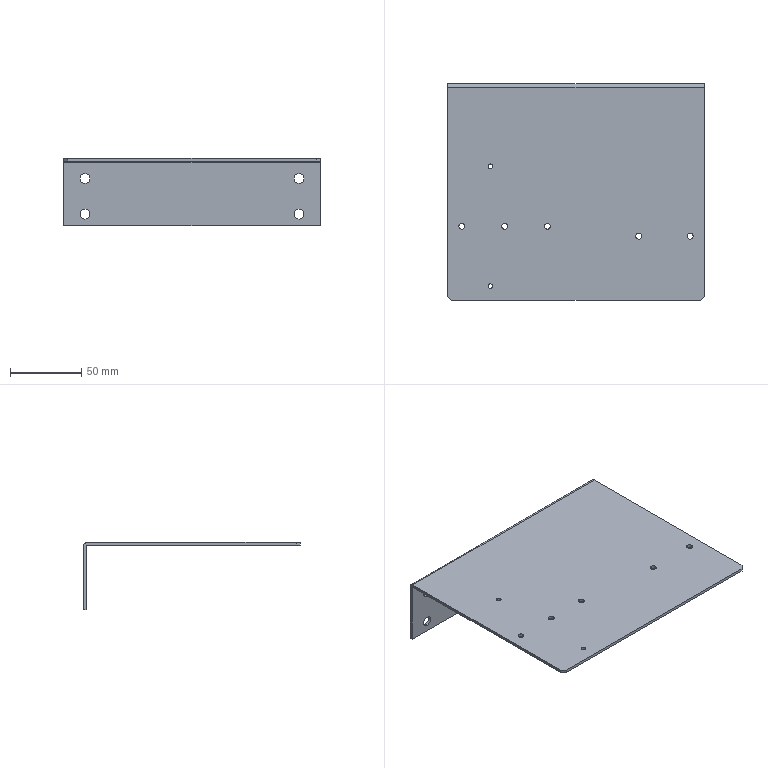Part | SolidWorks | features BaseBody 1 | 1 solid | 34 faces | box 180 x 152 x 47 mm | volume 70153 mm3 | cylinder 24 | plane 10 | commonest cylinder face diameters 4.2 x10 7 x8 3.3 x4 1.473 x1 5.473 x1
STEP:
#1=CARTESIAN_POINT('',(-80.,-100.1,2.));
#2=VERTEX_POINT('',#1);
#3=CARTESIAN_POINT('',(-80.,-95.9,2.));
#4=VERTEX_POINT('',#3);
#5=CARTESIAN_POINT('',(-80.,-98.,2.));
#6=DIRECTION('',(0.,0.,-1.));
#7=DIRECTION('',(0.,1.,0.));
#8=AXIS2_PLACEMENT_3D('',#5,#6,#7);
#9=CIRCLE('',#8,2.1);
#10=EDGE_CURVE('',#2,#4,#9,.T.);
#11=ORIENTED_EDGE('',*,*,#10,.F.);
#12=CARTESIAN_POINT('',(-80.,-100.1,0.));
#13=VERTEX_POINT('',#12);
#14=CARTESIAN_POINT('',(-80.,-100.1,0.));
#15=DIRECTION('',(0.,0.,-1.));
#16=VECTOR('',#15,1000.);
#17=LINE('',#14,#16);
#18=EDGE_CURVE('',#2,#13,#17,.T.);
#19=ORIENTED_EDGE('',*,*,#18,.T.);
#20=CARTESIAN_POINT('',(-80.,-95.9,0.));
#21=VERTEX_POINT('',#20);
#22=CARTESIAN_POINT('',(-80.,-98.,0.));
#23=DIRECTION('',(0.,0.,-1.));
#24=DIRECTION('',(0.,1.,0.));
#25=AXIS2_PLACEMENT_3D('',#22,#23,#24);
#26=CIRCLE('',#25,2.1);
#27=EDGE_CURVE('',#13,#21,#26,.T.);
#28=ORIENTED_EDGE('',*,*,#27,.T.);
#29=CARTESIAN_POINT('',(-80.,-95.9,0.));
#30=DIRECTION('',(0.,0.,-1.));
#31=VECTOR('',#30,1000.);
#32=LINE('',#29,#31);
#33=EDGE_CURVE('',#4,#21,#32,.T.);
#34=ORIENTED_EDGE('',*,*,#33,.F.);
#35=EDGE_LOOP('',(#11,#19,#28,#34));
#36=FACE_OUTER_BOUND('',#35,.T.);
#37=CARTESIAN_POINT('',(-80.,-98.,0.));
#38=DIRECTION('',(0.,0.,-1.));
#39=DIRECTION('',(0.,1.,0.));
#40=AXIS2_PLACEMENT_3D('',#37,#38,#39);
#41=CYLINDRICAL_SURFACE('',#40,2.1);
#42=ADVANCED_FACE('',(#36),#41,.F.);
#43=CARTESIAN_POINT('',(-50.,-100.1,2.));
#44=VERTEX_POINT('',#43);
#45=CARTESIAN_POINT('',(-50.,-95.9,2.));
#46=VERTEX_POINT('',#45);
#47=CARTESIAN_POINT('',(-50.,-98.,2.));
#48=DIRECTION('',(0.,0.,-1.));
#49=DIRECTION('',(0.,1.,0.));
#50=AXIS2_PLACEMENT_3D('',#47,#48,#49);
#51=CIRCLE('',#50,2.1);
#52=EDGE_CURVE('',#44,#46,#51,.T.);
#53=ORIENTED_EDGE('',*,*,#52,.F.);
#54=CARTESIAN_POINT('',(-50.,-100.1,0.));
#55=VERTEX_POINT('',#54);
#56=CARTESIAN_POINT('',(-50.,-100.1,0.));
#57=DIRECTION('',(0.,0.,-1.));
#58=VECTOR('',#57,1000.);
#59=LINE('',#56,#58);
#60=EDGE_CURVE('',#44,#55,#59,.T.);
#61=ORIENTED_EDGE('',*,*,#60,.T.);
#62=CARTESIAN_POINT('',(-50.,-95.9,0.));
#63=VERTEX_POINT('',#62);
#64=CARTESIAN_POINT('',(-50.,-98.,0.));
#65=DIRECTION('',(0.,0.,-1.));
#66=DIRECTION('',(0.,1.,0.));
#67=AXIS2_PLACEMENT_3D('',#64,#65,#66);
#68=CIRCLE('',#67,2.1);
#69=EDGE_CURVE('',#55,#63,#68,.T.);
#70=ORIENTED_EDGE('',*,*,#69,.T.);
#71=CARTESIAN_POINT('',(-50.,-95.9,0.));
#72=DIRECTION('',(0.,0.,-1.));
#73=VECTOR('',#72,1000.);
#74=LINE('',#71,#73);
#75=EDGE_CURVE('',#46,#63,#74,.T.);
#76=ORIENTED_EDGE('',*,*,#75,.F.);
#77=EDGE_LOOP('',(#53,#61,#70,#76));
#78=FACE_OUTER_BOUND('',#77,.T.);
#79=CARTESIAN_POINT('',(-50.,-98.,0.));
#80=DIRECTION('',(0.,0.,-1.));
#81=DIRECTION('',(0.,1.,0.));
#82=AXIS2_PLACEMENT_3D('',#79,#80,#81);
#83=CYLINDRICAL_SURFACE('',#82,2.1);
#84=ADVANCED_FACE('',(#78),#83,.F.);
#85=CARTESIAN_POINT('',(-20.,-100.1,2.));
#86=VERTEX_POINT('',#85);
#87=CARTESIAN_POINT('',(-20.,-95.9,2.));
#88=VERTEX_POINT('',#87);
#89=CARTESIAN_POINT('',(-20.,-98.,2.));
#90=DIRECTION('',(0.,0.,-1.));
#91=DIRECTION('',(0.,1.,0.));
#92=AXIS2_PLACEMENT_3D('',#89,#90,#91);
#93=CIRCLE('',#92,2.1);
#94=EDGE_CURVE('',#86,#88,#93,.T.);
#95=ORIENTED_EDGE('',*,*,#94,.F.);
#96=CARTESIAN_POINT('',(-20.,-100.1,0.));
#97=VERTEX_POINT('',#96);
#98=CARTESIAN_POINT('',(-20.,-100.1,0.));
#99=DIRECTION('',(0.,0.,-1.));
#100=VECTOR('',#99,1000.);
#101=LINE('',#98,#100);
#102=EDGE_CURVE('',#86,#97,#101,.T.);
#103=ORIENTED_EDGE('',*,*,#102,.T.);
#104=CARTESIAN_POINT('',(-20.,-95.9,0.));
#105=VERTEX_POINT('',#104);
#106=CARTESIAN_POINT('',(-20.,-98.,0.));
#107=DIRECTION('',(0.,0.,-1.));
#108=DIRECTION('',(0.,1.,0.));
#109=AXIS2_PLACEMENT_3D('',#106,#107,#108);
#110=CIRCLE('',#109,2.1);
#111=EDGE_CURVE('',#97,#105,#110,.T.);
#112=ORIENTED_EDGE('',*,*,#111,.T.);
#113=CARTESIAN_POINT('',(-20.,-95.9,0.));
#114=DIRECTION('',(0.,0.,-1.));
#115=VECTOR('',#114,1000.);
#116=LINE('',#113,#115);
#117=EDGE_CURVE('',#88,#105,#116,.T.);
#118=ORIENTED_EDGE('',*,*,#117,.F.);
#119=EDGE_LOOP('',(#95,#103,#112,#118));
#120=FACE_OUTER_BOUND('',#119,.T.);
#121=CARTESIAN_POINT('',(-20.,-98.,0.));
#122=DIRECTION('',(0.,0.,-1.));
#123=DIRECTION('',(0.,1.,0.));
#124=AXIS2_PLACEMENT_3D('',#121,#122,#123);
#125=CYLINDRICAL_SURFACE('',#124,2.1);
#126=ADVANCED_FACE('',(#120),#125,.F.);
#127=CARTESIAN_POINT('',(75.,0.,-33.5));
#128=VERTEX_POINT('',#127);
#129=CARTESIAN_POINT('',(75.,0.,-40.5));
#130=VERTEX_POINT('',#129);
#131=CARTESIAN_POINT('',(75.,0.,-37.));
#132=DIRECTION('',(0.,-1.,0.));
#133=DIRECTION('',(0.,0.,-1.));
#134=AXIS2_PLACEMENT_3D('',#131,#132,#133);
#135=CIRCLE('',#134,3.5);
#136=EDGE_CURVE('',#128,#130,#135,.T.);
#137=ORIENTED_EDGE('',*,*,#136,.T.);
#138=CARTESIAN_POINT('',(75.,2.,-40.5));
#139=VERTEX_POINT('',#138);
#140=CARTESIAN_POINT('',(75.,-8.,-40.5));
#141=DIRECTION('',(0.,1.,0.));
#142=VECTOR('',#141,1000.);
#143=LINE('',#140,#142);
#144=EDGE_CURVE('',#130,#139,#143,.T.);
#145=ORIENTED_EDGE('',*,*,#144,.T.);
#146=CARTESIAN_POINT('',(75.,2.,-33.5));
#147=VERTEX_POINT('',#146);
#148=CARTESIAN_POINT('',(75.,2.,-37.));
#149=DIRECTION('',(0.,1.,0.));
#150=DIRECTION('',(0.,0.,-1.));
#151=AXIS2_PLACEMENT_3D('',#148,#149,#150);
#152=CIRCLE('',#151,3.5);
#153=EDGE_CURVE('',#139,#147,#152,.T.);
#154=ORIENTED_EDGE('',*,*,#153,.T.);
#155=CARTESIAN_POINT('',(75.,-8.,-33.5));
#156=DIRECTION('',(0.,1.,0.));
#157=VECTOR('',#156,1000.);
#158=LINE('',#155,#157);
#159=EDGE_CURVE('',#128,#147,#158,.T.);
#160=ORIENTED_EDGE('',*,*,#159,.F.);
#161=EDGE_LOOP('',(#137,#145,#154,#160));
#162=FACE_OUTER_BOUND('',#161,.T.);
#163=CARTESIAN_POINT('',(75.,-8.,-37.));
#164=DIRECTION('',(0.,1.,0.));
#165=DIRECTION('',(0.,0.,1.));
#166=AXIS2_PLACEMENT_3D('',#163,#164,#165);
#167=CYLINDRICAL_SURFACE('',#166,3.5);
#168=ADVANCED_FACE('',(#162),#167,.F.);
#169=CARTESIAN_POINT('',(75.,0.,-8.5));
#170=VERTEX_POINT('',#169);
#171=CARTESIAN_POINT('',(75.,0.,-15.5));
#172=VERTEX_POINT('',#171);
#173=CARTESIAN_POINT('',(75.,0.,-12.));
#174=DIRECTION('',(0.,-1.,0.));
#175=DIRECTION('',(0.,0.,-1.));
#176=AXIS2_PLACEMENT_3D('',#173,#174,#175);
#177=CIRCLE('',#176,3.5);
#178=EDGE_CURVE('',#170,#172,#177,.T.);
#179=ORIENTED_EDGE('',*,*,#178,.T.);
#180=CARTESIAN_POINT('',(75.,2.,-15.5));
#181=VERTEX_POINT('',#180);
#182=CARTESIAN_POINT('',(75.,-8.,-15.5));
#183=DIRECTION('',(0.,1.,0.));
#184=VECTOR('',#183,1000.);
#185=LINE('',#182,#184);
#186=EDGE_CURVE('',#172,#181,#185,.T.);
#187=ORIENTED_EDGE('',*,*,#186,.T.);
#188=CARTESIAN_POINT('',(75.,2.,-8.5));
#189=VERTEX_POINT('',#188);
#190=CARTESIAN_POINT('',(75.,2.,-12.));
#191=DIRECTION('',(0.,1.,0.));
#192=DIRECTION('',(0.,0.,1.));
#193=AXIS2_PLACEMENT_3D('',#190,#191,#192);
#194=CIRCLE('',#193,3.5);
#195=EDGE_CURVE('',#181,#189,#194,.T.);
#196=ORIENTED_EDGE('',*,*,#195,.T.);
#197=CARTESIAN_POINT('',(75.,-8.,-8.5));
#198=DIRECTION('',(0.,1.,0.));
#199=VECTOR('',#198,1000.);
#200=LINE('',#197,#199);
#201=EDGE_CURVE('',#170,#189,#200,.T.);
#202=ORIENTED_EDGE('',*,*,#201,.F.);
#203=EDGE_LOOP('',(#179,#187,#196,#202));
#204=FACE_OUTER_BOUND('',#203,.T.);
#205=CARTESIAN_POINT('',(75.,-8.,-12.));
#206=DIRECTION('',(0.,1.,0.));
#207=DIRECTION('',(0.,0.,1.));
#208=AXIS2_PLACEMENT_3D('',#205,#206,#207);
#209=CYLINDRICAL_SURFACE('',#208,3.5);
#210=ADVANCED_FACE('',(#204),#209,.F.);
#211=CARTESIAN_POINT('',(-75.,0.,-8.5));
#212=VERTEX_POINT('',#211);
#213=CARTESIAN_POINT('',(-75.,0.,-15.5));
#214=VERTEX_POINT('',#213);
#215=CARTESIAN_POINT('',(-75.,0.,-12.));
#216=DIRECTION('',(0.,-1.,0.));
#217=DIRECTION('',(0.,0.,-1.));
#218=AXIS2_PLACEMENT_3D('',#215,#216,#217);
#219=CIRCLE('',#218,3.5);
#220=EDGE_CURVE('',#212,#214,#219,.T.);
#221=ORIENTED_EDGE('',*,*,#220,.T.);
#222=CARTESIAN_POINT('',(-75.,2.,-15.5));
#223=VERTEX_POINT('',#222);
#224=CARTESIAN_POINT('',(-75.,-8.,-15.5));
#225=DIRECTION('',(0.,1.,0.));
#226=VECTOR('',#225,1000.);
#227=LINE('',#224,#226);
#228=EDGE_CURVE('',#214,#223,#227,.T.);
#229=ORIENTED_EDGE('',*,*,#228,.T.);
#230=CARTESIAN_POINT('',(-75.,2.,-8.5));
#231=VERTEX_POINT('',#230);
#232=CARTESIAN_POINT('',(-75.,2.,-12.));
#233=DIRECTION('',(0.,1.,0.));
#234=DIRECTION('',(0.,0.,-1.));
#235=AXIS2_PLACEMENT_3D('',#232,#233,#234);
#236=CIRCLE('',#235,3.5);
#237=EDGE_CURVE('',#223,#231,#236,.T.);
#238=ORIENTED_EDGE('',*,*,#237,.T.);
#239=CARTESIAN_POINT('',(-75.,-8.,-8.5));
#240=DIRECTION('',(0.,1.,0.));
#241=VECTOR('',#240,1000.);
#242=LINE('',#239,#241);
#243=EDGE_CURVE('',#212,#231,#242,.T.);
#244=ORIENTED_EDGE('',*,*,#243,.F.);
#245=EDGE_LOOP('',(#221,#229,#238,#244));
#246=FACE_OUTER_BOUND('',#245,.T.);
#247=CARTESIAN_POINT('',(-75.,-8.,-12.));
#248=DIRECTION('',(0.,1.,0.));
#249=DIRECTION('',(0.,0.,1.));
#250=AXIS2_PLACEMENT_3D('',#247,#248,#249);
#251=CYLINDRICAL_SURFACE('',#250,3.5);
#252=ADVANCED_FACE('',(#246),#251,.F.);
#253=CARTESIAN_POINT('',(-75.,0.,-33.5));
#254=VERTEX_POINT('',#253);
#255=CARTESIAN_POINT('',(-75.,0.,-40.5));
#256=VERTEX_POINT('',#255);
#257=CARTESIAN_POINT('',(-75.,0.,-37.));
#258=DIRECTION('',(0.,-1.,0.));
#259=DIRECTION('',(0.,0.,-1.));
#260=AXIS2_PLACEMENT_3D('',#257,#258,#259);
#261=CIRCLE('',#260,3.5);
#262=EDGE_CURVE('',#254,#256,#261,.T.);
#263=ORIENTED_EDGE('',*,*,#262,.T.);
#264=CARTESIAN_POINT('',(-75.,2.,-40.5));
#265=VERTEX_POINT('',#264);
#266=CARTESIAN_POINT('',(-75.,-8.,-40.5));
#267=DIRECTION('',(0.,1.,0.));
#268=VECTOR('',#267,1000.);
#269=LINE('',#266,#268);
#270=EDGE_CURVE('',#256,#265,#269,.T.);
#271=ORIENTED_EDGE('',*,*,#270,.T.);
#272=CARTESIAN_POINT('',(-75.,2.,-33.5));
#273=VERTEX_POINT('',#272);
#274=CARTESIAN_POINT('',(-75.,2.,-37.));
#275=DIRECTION('',(0.,1.,0.));
#276=DIRECTION('',(0.,0.,1.));
#277=AXIS2_PLACEMENT_3D('',#274,#275,#276);
#278=CIRCLE('',#277,3.5);
#279=EDGE_CURVE('',#265,#273,#278,.T.);
#280=ORIENTED_EDGE('',*,*,#279,.T.);
#281=CARTESIAN_POINT('',(-75.,-8.,-33.5));
#282=DIRECTION('',(0.,1.,0.));
#283=VECTOR('',#282,1000.);
#284=LINE('',#281,#283);
#285=EDGE_CURVE('',#254,#273,#284,.T.);
#286=ORIENTED_EDGE('',*,*,#285,.F.);
#287=EDGE_LOOP('',(#263,#271,#280,#286));
#288=FACE_OUTER_BOUND('',#287,.T.);
#289=CARTESIAN_POINT('',(-75.,-8.,-37.));
#290=DIRECTION('',(0.,1.,0.));
#291=DIRECTION('',(0.,0.,1.));
#292=AXIS2_PLACEMENT_3D('',#289,#290,#291);
#293=CYLINDRICAL_SURFACE('',#292,3.5);
#294=ADVANCED_FACE('',(#288),#293,.F.);
#295=CARTESIAN_POINT('',(-60.,-57.65,2.));
#296=VERTEX_POINT('',#295);
#297=CARTESIAN_POINT('',(-60.,-54.35,2.));
#298=VERTEX_POINT('',#297);
#299=CARTESIAN_POINT('',(-60.,-56.,2.));
#300=DIRECTION('',(0.,0.,-1.));
#301=DIRECTION('',(0.,1.,0.));
#302=AXIS2_PLACEMENT_3D('',#299,#300,#301);
#303=CIRCLE('',#302,1.65);
#304=EDGE_CURVE('',#296,#298,#303,.T.);
#305=ORIENTED_EDGE('',*,*,#304,.F.);
#306=CARTESIAN_POINT('',(-60.,-57.65,0.));
#307=VERTEX_POINT('',#306);
#308=CARTESIAN_POINT('',(-60.,-57.65,0.));
#309=DIRECTION('',(0.,0.,-1.));
#310=VECTOR('',#309,1000.);
#311=LINE('',#308,#310);
#312=EDGE_CURVE('',#296,#307,#311,.T.);
#313=ORIENTED_EDGE('',*,*,#312,.T.);
#314=CARTESIAN_POINT('',(-60.,-54.35,0.));
#315=VERTEX_POINT('',#314);
#316=CARTESIAN_POINT('',(-60.,-56.,0.));
#317=DIRECTION('',(0.,0.,-1.));
#318=DIRECTION('',(0.,1.,0.));
#319=AXIS2_PLACEMENT_3D('',#316,#317,#318);
#320=CIRCLE('',#319,1.65);
#321=EDGE_CURVE('',#307,#315,#320,.T.);
#322=ORIENTED_EDGE('',*,*,#321,.T.);
#323=CARTESIAN_POINT('',(-60.,-54.35,0.));
#324=DIRECTION('',(0.,0.,-1.));
#325=VECTOR('',#324,1000.);
#326=LINE('',#323,#325);
#327=EDGE_CURVE('',#298,#315,#326,.T.);
#328=ORIENTED_EDGE('',*,*,#327,.F.);
#329=EDGE_LOOP('',(#305,#313,#322,#328));
#330=FACE_OUTER_BOUND('',#329,.T.);
#331=CARTESIAN_POINT('',(-60.,-56.,0.));
#332=DIRECTION('',(0.,0.,-1.));
#333=DIRECTION('',(0.,1.,0.));
#334=AXIS2_PLACEMENT_3D('',#331,#332,#333);
#335=CYLINDRICAL_SURFACE('',#334,1.65);
#336=ADVANCED_FACE('',(#330),#335,.F.);
#337=CARTESIAN_POINT('',(-60.,-141.65,2.));
#338=VERTEX_POINT('',#337);
#339=CARTESIAN_POINT('',(-60.,-138.35,2.));
#340=VERTEX_POINT('',#339);
#341=CARTESIAN_POINT('',(-60.,-140.,2.));
#342=DIRECTION('',(0.,0.,-1.));
#343=DIRECTION('',(0.,1.,0.));
#344=AXIS2_PLACEMENT_3D('',#341,#342,#343);
#345=CIRCLE('',#344,1.65);
#346=EDGE_CURVE('',#338,#340,#345,.T.);
#347=ORIENTED_EDGE('',*,*,#346,.F.);
#348=CARTESIAN_POINT('',(-60.,-141.65,0.));
#349=VERTEX_POINT('',#348);
#350=CARTESIAN_POINT('',(-60.,-141.65,0.));
#351=DIRECTION('',(0.,0.,-1.));
#352=VECTOR('',#351,1000.);
#353=LINE('',#350,#352);
#354=EDGE_CURVE('',#338,#349,#353,.T.);
#355=ORIENTED_EDGE('',*,*,#354,.T.);
#356=CARTESIAN_POINT('',(-60.,-138.35,0.));
#357=VERTEX_POINT('',#356);
#358=CARTESIAN_POINT('',(-60.,-140.,0.));
#359=DIRECTION('',(0.,0.,-1.));
#360=DIRECTION('',(0.,1.,0.));
#361=AXIS2_PLACEMENT_3D('',#358,#359,#360);
#362=CIRCLE('',#361,1.65);
#363=EDGE_CURVE('',#349,#357,#362,.T.);
#364=ORIENTED_EDGE('',*,*,#363,.T.);
#365=CARTESIAN_POINT('',(-60.,-138.35,0.));
#366=DIRECTION('',(0.,0.,-1.));
#367=VECTOR('',#366,1000.);
#368=LINE('',#365,#367);
#369=EDGE_CURVE('',#340,#357,#368,.T.);
#370=ORIENTED_EDGE('',*,*,#369,.F.);
#371=EDGE_LOOP('',(#347,#355,#364,#370));
#372=FACE_OUTER_BOUND('',#371,.T.);
#373=CARTESIAN_POINT('',(-60.,-140.,0.));
#374=DIRECTION('',(0.,0.,-1.));
#375=DIRECTION('',(0.,1.,0.));
#376=AXIS2_PLACEMENT_3D('',#373,#374,#375);
#377=CYLINDRICAL_SURFACE('',#376,1.65);
#378=ADVANCED_FACE('',(#372),#377,.F.);
#379=CARTESIAN_POINT('',(80.,-107.1,2.));
#380=VERTEX_POINT('',#379);
#381=CARTESIAN_POINT('',(80.,-102.9,2.));
#382=VERTEX_POINT('',#381);
#383=CARTESIAN_POINT('',(80.,-105.,2.));
#384=DIRECTION('',(0.,0.,-1.));
#385=DIRECTION('',(0.,1.,0.));
#386=AXIS2_PLACEMENT_3D('',#383,#384,#385);
#387=CIRCLE('',#386,2.1);
#388=EDGE_CURVE('',#380,#382,#387,.T.);
#389=ORIENTED_EDGE('',*,*,#388,.F.);
#390=CARTESIAN_POINT('',(80.,-107.1,0.));
#391=VERTEX_POINT('',#390);
#392=CARTESIAN_POINT('',(80.,-107.1,0.));
#393=DIRECTION('',(0.,0.,-1.));
#394=VECTOR('',#393,1000.);
#395=LINE('',#392,#394);
#396=EDGE_CURVE('',#380,#391,#395,.T.);
#397=ORIENTED_EDGE('',*,*,#396,.T.);
#398=CARTESIAN_POINT('',(80.,-102.9,0.));
#399=VERTEX_POINT('',#398);
#400=CARTESIAN_POINT('',(80.,-105.,0.));
#401=DIRECTION('',(0.,0.,-1.));
#402=DIRECTION('',(0.,1.,0.));
#403=AXIS2_PLACEMENT_3D('',#400,#401,#402);
#404=CIRCLE('',#403,2.1);
#405=EDGE_CURVE('',#391,#399,#404,.T.);
#406=ORIENTED_EDGE('',*,*,#405,.T.);
#407=CARTESIAN_POINT('',(80.,-102.9,0.));
#408=DIRECTION('',(0.,0.,-1.));
#409=VECTOR('',#408,1000.);
#410=LINE('',#407,#409);
#411=EDGE_CURVE('',#382,#399,#410,.T.);
#412=ORIENTED_EDGE('',*,*,#411,.F.);
#413=EDGE_LOOP('',(#389,#397,#406,#412));
#414=FACE_OUTER_BOUND('',#413,.T.);
#415=CARTESIAN_POINT('',(80.,-105.,0.));
#416=DIRECTION('',(0.,0.,-1.));
#417=DIRECTION('',(0.,1.,0.));
#418=AXIS2_PLACEMENT_3D('',#415,#416,#417);
#419=CYLINDRICAL_SURFACE('',#418,2.1);
#420=ADVANCED_FACE('',(#414),#419,.F.);
#421=CARTESIAN_POINT('',(44.,-107.1,2.));
#422=VERTEX_POINT('',#421);
#423=CARTESIAN_POINT('',(44.,-102.9,2.));
#424=VERTEX_POINT('',#423);
#425=CARTESIAN_POINT('',(44.,-105.,2.));
#426=DIRECTION('',(0.,0.,-1.));
#427=DIRECTION('',(0.,1.,0.));
#428=AXIS2_PLACEMENT_3D('',#425,#426,#427);
#429=CIRCLE('',#428,2.1);
#430=EDGE_CURVE('',#422,#424,#429,.T.);
#431=ORIENTED_EDGE('',*,*,#430,.F.);
#432=CARTESIAN_POINT('',(44.,-107.1,0.));
#433=VERTEX_POINT('',#432);
#434=CARTESIAN_POINT('',(44.,-107.1,0.));
#435=DIRECTION('',(0.,0.,-1.));
#436=VECTOR('',#435,1000.);
#437=LINE('',#434,#436);
#438=EDGE_CURVE('',#422,#433,#437,.T.);
#439=ORIENTED_EDGE('',*,*,#438,.T.);
#440=CARTESIAN_POINT('',(44.,-102.9,0.));
#441=VERTEX_POINT('',#440);
#442=CARTESIAN_POINT('',(44.,-105.,0.));
#443=DIRECTION('',(0.,0.,-1.));
#444=DIRECTION('',(0.,1.,0.));
#445=AXIS2_PLACEMENT_3D('',#442,#443,#444);
#446=CIRCLE('',#445,2.1);
#447=EDGE_CURVE('',#433,#441,#446,.T.);
#448=ORIENTED_EDGE('',*,*,#447,.T.);
#449=CARTESIAN_POINT('',(44.,-102.9,0.));
#450=DIRECTION('',(0.,0.,-1.));
#451=VECTOR('',#450,1000.);
#452=LINE('',#449,#451);
#453=EDGE_CURVE('',#424,#441,#452,.T.);
#454=ORIENTED_EDGE('',*,*,#453,.F.);
#455=EDGE_LOOP('',(#431,#439,#448,#454));
#456=FACE_OUTER_BOUND('',#455,.T.);
#457=CARTESIAN_POINT('',(44.,-105.,0.));
#458=DIRECTION('',(0.,0.,-1.));
#459=DIRECTION('',(0.,1.,0.));
#460=AXIS2_PLACEMENT_3D('',#457,#458,#459);
#461=CYLINDRICAL_SURFACE('',#460,2.1);
#462=ADVANCED_FACE('',(#456),#461,.F.);
#463=CARTESIAN_POINT('',(-87.,-150.,0.));
#464=VERTEX_POINT('',#463);
#465=CARTESIAN_POINT('',(-90.,-147.,0.));
#466=VERTEX_POINT('',#465);
#467=CARTESIAN_POINT('',(-73.5,-163.5,0.));
#468=DIRECTION('',(-0.7071,0.7071,0.));
#469=VECTOR('',#468,1000.);
#470=LINE('',#467,#469);
#471=EDGE_CURVE('',#464,#466,#470,.T.);
#472=ORIENTED_EDGE('',*,*,#471,.F.);
#473=CARTESIAN_POINT('',(-87.,-150.,2.));
#474=VERTEX_POINT('',#473);
#475=CARTESIAN_POINT('',(-87.,-150.,0.));
#476=DIRECTION('',(0.,0.,-1.));
#477=VECTOR('',#476,1000.);
#478=LINE('',#475,#477);
#479=EDGE_CURVE('',#474,#464,#478,.T.);
#480=ORIENTED_EDGE('',*,*,#479,.F.);
#481=CARTESIAN_POINT('',(-90.,-147.,2.));
#482=VERTEX_POINT('',#481);
#483=CARTESIAN_POINT('',(-90.,-147.,2.));
#484=DIRECTION('',(0.7071,-0.7071,0.));
#485=VECTOR('',#484,1000.);
#486=LINE('',#483,#485);
#487=EDGE_CURVE('',#482,#474,#486,.T.);
#488=ORIENTED_EDGE('',*,*,#487,.F.);
#489=CARTESIAN_POINT('',(-90.,-147.,-0.7366));
#490=DIRECTION('',(0.,0.,1.));
#491=VECTOR('',#490,1000.);
#492=LINE('',#489,#491);
#493=EDGE_CURVE('',#466,#482,#492,.T.);
#494=ORIENTED_EDGE('',*,*,#493,.F.);
#495=EDGE_LOOP('',(#472,#480,#488,#494));
#496=FACE_OUTER_BOUND('',#495,.T.);
#497=CARTESIAN_POINT('',(-90.,-147.,-0.7366));
#498=DIRECTION('',(0.7071,0.7071,0.));
#499=DIRECTION('',(0.,0.,-1.));
#500=AXIS2_PLACEMENT_3D('',#497,#498,#499);
#501=PLANE('',#500);
#502=ADVANCED_FACE('',(#496),#501,.F.);
#503=CARTESIAN_POINT('',(90.,-147.,0.));
#504=VERTEX_POINT('',#503);
#505=CARTESIAN_POINT('',(87.,-150.,0.));
#506=VERTEX_POINT('',#505);
#507=CARTESIAN_POINT('',(163.5,-73.5,0.));
#508=DIRECTION('',(-0.7071,-0.7071,0.));
#509=VECTOR('',#508,1000.);
#510=LINE('',#507,#509);
#511=EDGE_CURVE('',#504,#506,#510,.T.);
#512=ORIENTED_EDGE('',*,*,#511,.F.);
#513=CARTESIAN_POINT('',(90.,-147.,2.));
#514=VERTEX_POINT('',#513);
#515=CARTESIAN_POINT('',(90.,-147.,-0.7366));
#516=DIRECTION('',(0.,0.,-1.));
#517=VECTOR('',#516,1000.);
#518=LINE('',#515,#517);
#519=EDGE_CURVE('',#514,#504,#518,.T.);
#520=ORIENTED_EDGE('',*,*,#519,.F.);
#521=CARTESIAN_POINT('',(87.,-150.,2.));
#522=VERTEX_POINT('',#521);
#523=CARTESIAN_POINT('',(87.,-150.,2.));
#524=DIRECTION('',(0.7071,0.7071,0.));
#525=VECTOR('',#524,1000.);
#526=LINE('',#523,#525);
#527=EDGE_CURVE('',#522,#514,#526,.T.);
#528=ORIENTED_EDGE('',*,*,#527,.F.);
#529=CARTESIAN_POINT('',(87.,-150.,0.));
#530=DIRECTION('',(0.,0.,1.));
#531=VECTOR('',#530,1000.);
#532=LINE('',#529,#531);
#533=EDGE_CURVE('',#506,#522,#532,.T.);
#534=ORIENTED_EDGE('',*,*,#533,.F.);
#535=EDGE_LOOP('',(#512,#520,#528,#534));
#536=FACE_OUTER_BOUND('',#535,.T.);
#537=CARTESIAN_POINT('',(87.,-150.,0.));
#538=DIRECTION('',(-0.7071,0.7071,0.));
#539=DIRECTION('',(0.,0.,1.));
#540=AXIS2_PLACEMENT_3D('',#537,#538,#539);
#541=PLANE('',#540);
#542=ADVANCED_FACE('',(#536),#541,.F.);
#543=CARTESIAN_POINT('',(-90.,2.,-0.7366));
#544=VERTEX_POINT('',#543);
#545=CARTESIAN_POINT('',(-90.,-0.7366,2.));
#546=VERTEX_POINT('',#545);
#547=CARTESIAN_POINT('',(-90.,-0.7366,-0.7366));
#548=DIRECTION('',(1.,0.,0.));
#549=DIRECTION('',(0.,0.,-1.));
#550=AXIS2_PLACEMENT_3D('',#547,#548,#549);
#551=CIRCLE('',#550,2.737);
#552=EDGE_CURVE('',#544,#546,#551,.T.);
#553=ORIENTED_EDGE('',*,*,#552,.T.);
#554=CARTESIAN_POINT('',(90.,-0.7366,2.));
#555=VERTEX_POINT('',#554);
#556=CARTESIAN_POINT('',(90.,-0.7366,2.));
#557=DIRECTION('',(-1.,0.,0.));
#558=VECTOR('',#557,1000.);
#559=LINE('',#556,#558);
#560=EDGE_CURVE('',#555,#546,#559,.T.);
#561=ORIENTED_EDGE('',*,*,#560,.F.);
#562=CARTESIAN_POINT('',(90.,2.,-0.7366));
#563=VERTEX_POINT('',#562);
#564=CARTESIAN_POINT('',(90.,-0.7366,-0.7366));
#565=DIRECTION('',(1.,0.,0.));
#566=DIRECTION('',(0.,0.,-1.));
#567=AXIS2_PLACEMENT_3D('',#564,#565,#566);
#568=CIRCLE('',#567,2.737);
#569=EDGE_CURVE('',#563,#555,#568,.T.);
#570=ORIENTED_EDGE('',*,*,#569,.F.);
#571=CARTESIAN_POINT('',(90.,2.,-0.7366));
#572=DIRECTION('',(-1.,0.,0.));
#573=VECTOR('',#572,1000.);
#574=LINE('',#571,#573);
#575=EDGE_CURVE('',#563,#544,#574,.T.);
#576=ORIENTED_EDGE('',*,*,#575,.T.);
#577=EDGE_LOOP('',(#553,#561,#570,#576));
#578=FACE_OUTER_BOUND('',#577,.T.);
#579=CARTESIAN_POINT('',(90.,-0.7366,-0.7366));
#580=DIRECTION('',(-1.,0.,0.));
#581=DIRECTION('',(0.,0.,1.));
#582=AXIS2_PLACEMENT_3D('',#579,#580,#581);
#583=CYLINDRICAL_SURFACE('',#582,2.737);
#584=ADVANCED_FACE('',(#578),#583,.T.);
#585=CARTESIAN_POINT('',(-75.,2.,-37.));
#586=DIRECTION('',(0.,1.,0.));
#587=DIRECTION('',(0.,0.,1.));
#588=AXIS2_PLACEMENT_3D('',#585,#586,#587);
#589=CIRCLE('',#588,3.5);
#590=EDGE_CURVE('',#273,#265,#589,.T.);
#591=ORIENTED_EDGE('',*,*,#590,.F.);
#592=ORIENTED_EDGE('',*,*,#279,.F.);
#593=EDGE_LOOP('',(#591,#592));
#594=FACE_BOUND('',#593,.T.);
#595=CARTESIAN_POINT('',(-75.,2.,-12.));
#596=DIRECTION('',(0.,1.,0.));
#597=DIRECTION('',(0.,0.,-1.));
#598=AXIS2_PLACEMENT_3D('',#595,#596,#597);
#599=CIRCLE('',#598,3.5);
#600=EDGE_CURVE('',#231,#223,#599,.T.);
#601=ORIENTED_EDGE('',*,*,#600,.F.);
#602=ORIENTED_EDGE('',*,*,#237,.F.);
#603=EDGE_LOOP('',(#601,#602));
#604=FACE_BOUND('',#603,.T.);
#605=CARTESIAN_POINT('',(75.,2.,-12.));
#606=DIRECTION('',(0.,1.,0.));
#607=DIRECTION('',(0.,0.,1.));
#608=AXIS2_PLACEMENT_3D('',#605,#606,#607);
#609=CIRCLE('',#608,3.5);
#610=EDGE_CURVE('',#189,#181,#609,.T.);
#611=ORIENTED_EDGE('',*,*,#610,.F.);
#612=ORIENTED_EDGE('',*,*,#195,.F.);
#613=EDGE_LOOP('',(#611,#612));
#614=FACE_BOUND('',#613,.T.);
#615=CARTESIAN_POINT('',(75.,2.,-37.));
#616=DIRECTION('',(0.,1.,0.));
#617=DIRECTION('',(0.,0.,-1.));
#618=AXIS2_PLACEMENT_3D('',#615,#616,#617);
#619=CIRCLE('',#618,3.5);
#620=EDGE_CURVE('',#147,#139,#619,.T.);
#621=ORIENTED_EDGE('',*,*,#620,.F.);
#622=ORIENTED_EDGE('',*,*,#153,.F.);
#623=EDGE_LOOP('',(#621,#622));
#624=FACE_BOUND('',#623,.T.);
#625=CARTESIAN_POINT('',(-90.,2.,-45.));
#626=VERTEX_POINT('',#625);
#627=CARTESIAN_POINT('',(-90.,2.,-45.));
#628=DIRECTION('',(0.,0.,1.));
#629=VECTOR('',#628,1000.);
#630=LINE('',#627,#629);
#631=EDGE_CURVE('',#626,#544,#630,.T.);
#632=ORIENTED_EDGE('',*,*,#631,.T.);
#633=ORIENTED_EDGE('',*,*,#575,.F.);
#634=CARTESIAN_POINT('',(90.,2.,-45.));
#635=VERTEX_POINT('',#634);
#636=CARTESIAN_POINT('',(90.,2.,-45.));
#637=DIRECTION('',(0.,0.,1.));
#638=VECTOR('',#637,1000.);
#639=LINE('',#636,#638);
#640=EDGE_CURVE('',#635,#563,#639,.T.);
#641=ORIENTED_EDGE('',*,*,#640,.F.);
#642=CARTESIAN_POINT('',(90.,2.,-45.));
#643=DIRECTION('',(-1.,0.,0.));
#644=VECTOR('',#643,1000.);
#645=LINE('',#642,#644);
#646=EDGE_CURVE('',#635,#626,#645,.T.);
#647=ORIENTED_EDGE('',*,*,#646,.T.);
#648=EDGE_LOOP('',(#632,#633,#641,#647));
#649=FACE_OUTER_BOUND('',#648,.T.);
#650=CARTESIAN_POINT('',(90.,2.,-45.));
#651=DIRECTION('',(0.,-1.,0.));
#652=DIRECTION('',(-1.,0.,0.));
#653=AXIS2_PLACEMENT_3D('',#650,#651,#652);
#654=PLANE('',#653);
#655=ADVANCED_FACE('',(#594,#604,#614,#624,#649),#654,.F.);
#656=CARTESIAN_POINT('',(-90.,0.,-45.));
#657=VERTEX_POINT('',#656);
#658=CARTESIAN_POINT('',(-90.,2.,-45.));
#659=DIRECTION('',(0.,-1.,0.));
#660=VECTOR('',#659,1000.);
#661=LINE('',#658,#660);
#662=EDGE_CURVE('',#626,#657,#661,.T.);
#663=ORIENTED_EDGE('',*,*,#662,.F.);
#664=ORIENTED_EDGE('',*,*,#646,.F.);
#665=CARTESIAN_POINT('',(90.,0.,-45.));
#666=VERTEX_POINT('',#665);
#667=CARTESIAN_POINT('',(90.,2.,-45.));
#668=DIRECTION('',(0.,-1.,0.));
#669=VECTOR('',#668,1000.);
#670=LINE('',#667,#669);
#671=EDGE_CURVE('',#635,#666,#670,.T.);
#672=ORIENTED_EDGE('',*,*,#671,.T.);
#673=CARTESIAN_POINT('',(90.,0.,-45.));
#674=DIRECTION('',(-1.,0.,0.));
#675=VECTOR('',#674,1000.);
#676=LINE('',#673,#675);
#677=EDGE_CURVE('',#666,#657,#676,.T.);
#678=ORIENTED_EDGE('',*,*,#677,.T.);
#679=EDGE_LOOP('',(#663,#664,#672,#678));
#680=FACE_OUTER_BOUND('',#679,.T.);
#681=CARTESIAN_POINT('',(90.,2.,-45.));
#682=DIRECTION('',(0.,0.,-1.));
#683=DIRECTION('',(0.,-1.,0.));
#684=AXIS2_PLACEMENT_3D('',#681,#682,#683);
#685=PLANE('',#684);
#686=ADVANCED_FACE('',(#680),#685,.T.);
#687=ORIENTED_EDGE('',*,*,#262,.F.);
#688=CARTESIAN_POINT('',(-75.,0.,-37.));
#689=DIRECTION('',(0.,-1.,0.));
#690=DIRECTION('',(0.,0.,-1.));
#691=AXIS2_PLACEMENT_3D('',#688,#689,#690);
#692=CIRCLE('',#691,3.5);
#693=EDGE_CURVE('',#256,#254,#692,.T.);
#694=ORIENTED_EDGE('',*,*,#693,.F.);
#695=EDGE_LOOP('',(#687,#694));
#696=FACE_BOUND('',#695,.T.);
#697=ORIENTED_EDGE('',*,*,#220,.F.);
#698=CARTESIAN_POINT('',(-75.,0.,-12.));
#699=DIRECTION('',(0.,-1.,0.));
#700=DIRECTION('',(0.,0.,-1.));
#701=AXIS2_PLACEMENT_3D('',#698,#699,#700);
#702=CIRCLE('',#701,3.5);
#703=EDGE_CURVE('',#214,#212,#702,.T.);
#704=ORIENTED_EDGE('',*,*,#703,.F.);
#705=EDGE_LOOP('',(#697,#704));
#706=FACE_BOUND('',#705,.T.);
#707=ORIENTED_EDGE('',*,*,#178,.F.);
#708=CARTESIAN_POINT('',(75.,0.,-12.));
#709=DIRECTION('',(0.,-1.,0.));
#710=DIRECTION('',(0.,0.,-1.));
#711=AXIS2_PLACEMENT_3D('',#708,#709,#710);
#712=CIRCLE('',#711,3.5);
#713=EDGE_CURVE('',#172,#170,#712,.T.);
#714=ORIENTED_EDGE('',*,*,#713,.F.);
#715=EDGE_LOOP('',(#707,#714));
#716=FACE_BOUND('',#715,.T.);
#717=ORIENTED_EDGE('',*,*,#136,.F.);
#718=CARTESIAN_POINT('',(75.,0.,-37.));
#719=DIRECTION('',(0.,-1.,0.));
#720=DIRECTION('',(0.,0.,-1.));
#721=AXIS2_PLACEMENT_3D('',#718,#719,#720);
#722=CIRCLE('',#721,3.5);
#723=EDGE_CURVE('',#130,#128,#722,.T.);
#724=ORIENTED_EDGE('',*,*,#723,.F.);
#725=EDGE_LOOP('',(#717,#724));
#726=FACE_BOUND('',#725,.T.);
#727=CARTESIAN_POINT('',(-90.,0.,-0.7366));
#728=VERTEX_POINT('',#727);
#729=CARTESIAN_POINT('',(-90.,0.,-45.));
#730=DIRECTION('',(0.,0.,1.));
#731=VECTOR('',#730,1000.);
#732=LINE('',#729,#731);
#733=EDGE_CURVE('',#657,#728,#732,.T.);
#734=ORIENTED_EDGE('',*,*,#733,.F.);
#735=ORIENTED_EDGE('',*,*,#677,.F.);
#736=CARTESIAN_POINT('',(90.,0.,-0.7366));
#737=VERTEX_POINT('',#736);
#738=CARTESIAN_POINT('',(90.,0.,-45.));
#739=DIRECTION('',(0.,0.,1.));
#740=VECTOR('',#739,1000.);
#741=LINE('',#738,#740);
#742=EDGE_CURVE('',#666,#737,#741,.T.);
#743=ORIENTED_EDGE('',*,*,#742,.T.);
#744=CARTESIAN_POINT('',(90.,0.,-0.7366));
#745=DIRECTION('',(-1.,0.,0.));
#746=VECTOR('',#745,1000.);
#747=LINE('',#744,#746);
#748=EDGE_CURVE('',#737,#728,#747,.T.);
#749=ORIENTED_EDGE('',*,*,#748,.T.);
#750=EDGE_LOOP('',(#734,#735,#743,#749));
#751=FACE_OUTER_BOUND('',#750,.T.);
#752=CARTESIAN_POINT('',(90.,0.,-45.));
#753=DIRECTION('',(0.,-1.,0.));
#754=DIRECTION('',(-1.,0.,0.));
#755=AXIS2_PLACEMENT_3D('',#752,#753,#754);
#756=PLANE('',#755);
#757=ADVANCED_FACE('',(#696,#706,#716,#726,#751),#756,.T.);
#758=CARTESIAN_POINT('',(-90.,-0.7366,0.));
#759=VERTEX_POINT('',#758);
#760=CARTESIAN_POINT('',(-90.,-0.7366,-0.7366));
#761=DIRECTION('',(1.,0.,0.));
#762=DIRECTION('',(0.,0.,1.));
#763=AXIS2_PLACEMENT_3D('',#760,#761,#762);
#764=CIRCLE('',#763,0.7366);
#765=EDGE_CURVE('',#728,#759,#764,.T.);
#766=ORIENTED_EDGE('',*,*,#765,.F.);
#767=ORIENTED_EDGE('',*,*,#748,.F.);
#768=CARTESIAN_POINT('',(90.,-0.7366,0.));
#769=VERTEX_POINT('',#768);
#770=CARTESIAN_POINT('',(90.,-0.7366,-0.7366));
#771=DIRECTION('',(1.,0.,0.));
#772=DIRECTION('',(0.,0.,1.));
#773=AXIS2_PLACEMENT_3D('',#770,#771,#772);
#774=CIRCLE('',#773,0.7366);
#775=EDGE_CURVE('',#737,#769,#774,.T.);
#776=ORIENTED_EDGE('',*,*,#775,.T.);
#777=CARTESIAN_POINT('',(90.,-0.7366,0.));
#778=DIRECTION('',(-1.,0.,0.));
#779=VECTOR('',#778,1000.);
#780=LINE('',#777,#779);
#781=EDGE_CURVE('',#769,#759,#780,.T.);
#782=ORIENTED_EDGE('',*,*,#781,.T.);
#783=EDGE_LOOP('',(#766,#767,#776,#782));
#784=FACE_OUTER_BOUND('',#783,.T.);
#785=CARTESIAN_POINT('',(90.,-0.7366,-0.7366));
#786=DIRECTION('',(-1.,0.,0.));
#787=DIRECTION('',(0.,0.,1.));
#788=AXIS2_PLACEMENT_3D('',#785,#786,#787);
#789=CYLINDRICAL_SURFACE('',#788,0.7366);
#790=ADVANCED_FACE('',(#784),#789,.F.);
#791=CARTESIAN_POINT('',(44.,-105.,0.));
#792=DIRECTION('',(0.,0.,-1.));
#793=DIRECTION('',(0.,1.,0.));
#794=AXIS2_PLACEMENT_3D('',#791,#792,#793);
#795=CIRCLE('',#794,2.1);
#796=EDGE_CURVE('',#441,#433,#795,.T.);
#797=ORIENTED_EDGE('',*,*,#796,.F.);
#798=ORIENTED_EDGE('',*,*,#447,.F.);
#799=EDGE_LOOP('',(#797,#798));
#800=FACE_BOUND('',#799,.T.);
#801=CARTESIAN_POINT('',(80.,-105.,0.));
#802=DIRECTION('',(0.,0.,-1.));
#803=DIRECTION('',(0.,1.,0.));
#804=AXIS2_PLACEMENT_3D('',#801,#802,#803);
#805=CIRCLE('',#804,2.1);
#806=EDGE_CURVE('',#399,#391,#805,.T.);
#807=ORIENTED_EDGE('',*,*,#806,.F.);
#808=ORIENTED_EDGE('',*,*,#405,.F.);
#809=EDGE_LOOP('',(#807,#808));
#810=FACE_BOUND('',#809,.T.);
#811=CARTESIAN_POINT('',(-60.,-140.,0.));
#812=DIRECTION('',(0.,0.,-1.));
#813=DIRECTION('',(0.,1.,0.));
#814=AXIS2_PLACEMENT_3D('',#811,#812,#813);
#815=CIRCLE('',#814,1.65);
#816=EDGE_CURVE('',#357,#349,#815,.T.);
#817=ORIENTED_EDGE('',*,*,#816,.F.);
#818=ORIENTED_EDGE('',*,*,#363,.F.);
#819=EDGE_LOOP('',(#817,#818));
#820=FACE_BOUND('',#819,.T.);
#821=CARTESIAN_POINT('',(-60.,-56.,0.));
#822=DIRECTION('',(0.,0.,-1.));
#823=DIRECTION('',(0.,1.,0.));
#824=AXIS2_PLACEMENT_3D('',#821,#822,#823);
#825=CIRCLE('',#824,1.65);
#826=EDGE_CURVE('',#315,#307,#825,.T.);
#827=ORIENTED_EDGE('',*,*,#826,.F.);
#828=ORIENTED_EDGE('',*,*,#321,.F.);
#829=EDGE_LOOP('',(#827,#828));
#830=FACE_BOUND('',#829,.T.);
#831=CARTESIAN_POINT('',(-20.,-98.,0.));
#832=DIRECTION('',(0.,0.,-1.));
#833=DIRECTION('',(0.,1.,0.));
#834=AXIS2_PLACEMENT_3D('',#831,#832,#833);
#835=CIRCLE('',#834,2.1);
#836=EDGE_CURVE('',#105,#97,#835,.T.);
#837=ORIENTED_EDGE('',*,*,#836,.F.);
#838=ORIENTED_EDGE('',*,*,#111,.F.);
#839=EDGE_LOOP('',(#837,#838));
#840=FACE_BOUND('',#839,.T.);
#841=CARTESIAN_POINT('',(-50.,-98.,0.));
#842=DIRECTION('',(0.,0.,-1.));
#843=DIRECTION('',(0.,1.,0.));
#844=AXIS2_PLACEMENT_3D('',#841,#842,#843);
#845=CIRCLE('',#844,2.1);
#846=EDGE_CURVE('',#63,#55,#845,.T.);
#847=ORIENTED_EDGE('',*,*,#846,.F.);
#848=ORIENTED_EDGE('',*,*,#69,.F.);
#849=EDGE_LOOP('',(#847,#848));
#850=FACE_BOUND('',#849,.T.);
#851=CARTESIAN_POINT('',(-80.,-98.,0.));
#852=DIRECTION('',(0.,0.,-1.));
#853=DIRECTION('',(0.,1.,0.));
#854=AXIS2_PLACEMENT_3D('',#851,#852,#853);
#855=CIRCLE('',#854,2.1);
#856=EDGE_CURVE('',#21,#13,#855,.T.);
#857=ORIENTED_EDGE('',*,*,#856,.F.);
#858=ORIENTED_EDGE('',*,*,#27,.F.);
#859=EDGE_LOOP('',(#857,#858));
#860=FACE_BOUND('',#859,.T.);
#861=CARTESIAN_POINT('',(90.,0.,0.));
#862=DIRECTION('',(0.,-1.,0.));
#863=VECTOR('',#862,1000.);
#864=LINE('',#861,#863);
#865=EDGE_CURVE('',#769,#504,#864,.T.);
#866=ORIENTED_EDGE('',*,*,#865,.T.);
#867=ORIENTED_EDGE('',*,*,#511,.T.);
#868=CARTESIAN_POINT('',(90.,-150.,0.));
#869=DIRECTION('',(-1.,0.,0.));
#870=VECTOR('',#869,1000.);
#871=LINE('',#868,#870);
#872=EDGE_CURVE('',#506,#464,#871,.T.);
#873=ORIENTED_EDGE('',*,*,#872,.T.);
#874=ORIENTED_EDGE('',*,*,#471,.T.);
#875=CARTESIAN_POINT('',(-90.,0.,0.));
#876=DIRECTION('',(0.,-1.,0.));
#877=VECTOR('',#876,1000.);
#878=LINE('',#875,#877);
#879=EDGE_CURVE('',#759,#466,#878,.T.);
#880=ORIENTED_EDGE('',*,*,#879,.F.);
#881=ORIENTED_EDGE('',*,*,#781,.F.);
#882=EDGE_LOOP('',(#866,#867,#873,#874,#880,#881));
#883=FACE_OUTER_BOUND('',#882,.T.);
#884=CARTESIAN_POINT('',(90.,0.,0.));
#885=DIRECTION('',(0.,0.,-1.));
#886=DIRECTION('',(-1.,0.,0.));
#887=AXIS2_PLACEMENT_3D('',#884,#885,#886);
#888=PLANE('',#887);
#889=ADVANCED_FACE('',(#800,#810,#820,#830,#840,#850,#860,#883),#888,.T.);
#890=ORIENTED_EDGE('',*,*,#872,.F.);
#891=ORIENTED_EDGE('',*,*,#533,.T.);
#892=CARTESIAN_POINT('',(90.,-150.,2.));
#893=DIRECTION('',(-1.,0.,0.));
#894=VECTOR('',#893,1000.);
#895=LINE('',#892,#894);
#896=EDGE_CURVE('',#522,#474,#895,.T.);
#897=ORIENTED_EDGE('',*,*,#896,.T.);
#898=ORIENTED_EDGE('',*,*,#479,.T.);
#899=EDGE_LOOP('',(#890,#891,#897,#898));
#900=FACE_OUTER_BOUND('',#899,.T.);
#901=CARTESIAN_POINT('',(90.,-150.,0.));
#902=DIRECTION('',(0.,-1.,0.));
#903=DIRECTION('',(0.,0.,-1.));
#904=AXIS2_PLACEMENT_3D('',#901,#902,#903);
#905=PLANE('',#904);
#906=ADVANCED_FACE('',(#900),#905,.T.);
#907=CARTESIAN_POINT('',(44.,-105.,2.));
#908=DIRECTION('',(0.,0.,-1.));
#909=DIRECTION('',(0.,1.,0.));
#910=AXIS2_PLACEMENT_3D('',#907,#908,#909);
#911=CIRCLE('',#910,2.1);
#912=EDGE_CURVE('',#424,#422,#911,.T.);
#913=ORIENTED_EDGE('',*,*,#912,.T.);
#914=ORIENTED_EDGE('',*,*,#430,.T.);
#915=EDGE_LOOP('',(#913,#914));
#916=FACE_BOUND('',#915,.T.);
#917=CARTESIAN_POINT('',(80.,-105.,2.));
#918=DIRECTION('',(0.,0.,-1.));
#919=DIRECTION('',(0.,1.,0.));
#920=AXIS2_PLACEMENT_3D('',#917,#918,#919);
#921=CIRCLE('',#920,2.1);
#922=EDGE_CURVE('',#382,#380,#921,.T.);
#923=ORIENTED_EDGE('',*,*,#922,.T.);
#924=ORIENTED_EDGE('',*,*,#388,.T.);
#925=EDGE_LOOP('',(#923,#924));
#926=FACE_BOUND('',#925,.T.);
#927=CARTESIAN_POINT('',(-60.,-140.,2.));
#928=DIRECTION('',(0.,0.,-1.));
#929=DIRECTION('',(0.,1.,0.));
#930=AXIS2_PLACEMENT_3D('',#927,#928,#929);
#931=CIRCLE('',#930,1.65);
#932=EDGE_CURVE('',#340,#338,#931,.T.);
#933=ORIENTED_EDGE('',*,*,#932,.T.);
#934=ORIENTED_EDGE('',*,*,#346,.T.);
#935=EDGE_LOOP('',(#933,#934));
#936=FACE_BOUND('',#935,.T.);
#937=CARTESIAN_POINT('',(-60.,-56.,2.));
#938=DIRECTION('',(0.,0.,-1.));
#939=DIRECTION('',(0.,1.,0.));
#940=AXIS2_PLACEMENT_3D('',#937,#938,#939);
#941=CIRCLE('',#940,1.65);
#942=EDGE_CURVE('',#298,#296,#941,.T.);
#943=ORIENTED_EDGE('',*,*,#942,.T.);
#944=ORIENTED_EDGE('',*,*,#304,.T.);
#945=EDGE_LOOP('',(#943,#944));
#946=FACE_BOUND('',#945,.T.);
#947=CARTESIAN_POINT('',(-20.,-98.,2.));
#948=DIRECTION('',(0.,0.,-1.));
#949=DIRECTION('',(0.,1.,0.));
#950=AXIS2_PLACEMENT_3D('',#947,#948,#949);
#951=CIRCLE('',#950,2.1);
#952=EDGE_CURVE('',#88,#86,#951,.T.);
#953=ORIENTED_EDGE('',*,*,#952,.T.);
#954=ORIENTED_EDGE('',*,*,#94,.T.);
#955=EDGE_LOOP('',(#953,#954));
#956=FACE_BOUND('',#955,.T.);
#957=CARTESIAN_POINT('',(-50.,-98.,2.));
#958=DIRECTION('',(0.,0.,-1.));
#959=DIRECTION('',(0.,1.,0.));
#960=AXIS2_PLACEMENT_3D('',#957,#958,#959);
#961=CIRCLE('',#960,2.1);
#962=EDGE_CURVE('',#46,#44,#961,.T.);
#963=ORIENTED_EDGE('',*,*,#962,.T.);
#964=ORIENTED_EDGE('',*,*,#52,.T.);
#965=EDGE_LOOP('',(#963,#964));
#966=FACE_BOUND('',#965,.T.);
#967=CARTESIAN_POINT('',(-80.,-98.,2.));
#968=DIRECTION('',(0.,0.,-1.));
#969=DIRECTION('',(0.,1.,0.));
#970=AXIS2_PLACEMENT_3D('',#967,#968,#969);
#971=CIRCLE('',#970,2.1);
#972=EDGE_CURVE('',#4,#2,#971,.T.);
#973=ORIENTED_EDGE('',*,*,#972,.T.);
#974=ORIENTED_EDGE('',*,*,#10,.T.);
#975=EDGE_LOOP('',(#973,#974));
#976=FACE_BOUND('',#975,.T.);
#977=ORIENTED_EDGE('',*,*,#896,.F.);
#978=ORIENTED_EDGE('',*,*,#527,.T.);
#979=CARTESIAN_POINT('',(90.,0.,2.));
#980=DIRECTION('',(0.,-1.,0.));
#981=VECTOR('',#980,1000.);
#982=LINE('',#979,#981);
#983=EDGE_CURVE('',#555,#514,#982,.T.);
#984=ORIENTED_EDGE('',*,*,#983,.F.);
#985=ORIENTED_EDGE('',*,*,#560,.T.);
#986=CARTESIAN_POINT('',(-90.,0.,2.));
#987=DIRECTION('',(0.,-1.,0.));
#988=VECTOR('',#987,1000.);
#989=LINE('',#986,#988);
#990=EDGE_CURVE('',#546,#482,#989,.T.);
#991=ORIENTED_EDGE('',*,*,#990,.T.);
#992=ORIENTED_EDGE('',*,*,#487,.T.);
#993=EDGE_LOOP('',(#977,#978,#984,#985,#991,#992));
#994=FACE_OUTER_BOUND('',#993,.T.);
#995=CARTESIAN_POINT('',(90.,0.,2.));
#996=DIRECTION('',(0.,0.,-1.));
#997=DIRECTION('',(-1.,0.,0.));
#998=AXIS2_PLACEMENT_3D('',#995,#996,#997);
#999=PLANE('',#998);
#1000=ADVANCED_FACE('',(#916,#926,#936,#946,#956,#966,#976,#994),#999,.F.);
#1001=ORIENTED_EDGE('',*,*,#552,.F.);
#1002=ORIENTED_EDGE('',*,*,#631,.F.);
#1003=ORIENTED_EDGE('',*,*,#662,.T.);
#1004=ORIENTED_EDGE('',*,*,#733,.T.);
#1005=ORIENTED_EDGE('',*,*,#765,.T.);
#1006=ORIENTED_EDGE('',*,*,#879,.T.);
#1007=ORIENTED_EDGE('',*,*,#493,.T.);
#1008=ORIENTED_EDGE('',*,*,#990,.F.);
#1009=EDGE_LOOP('',(#1001,#1002,#1003,#1004,#1005,#1006,#1007,#1008));
#1010=FACE_OUTER_BOUND('',#1009,.T.);
#1011=CARTESIAN_POINT('',(-90.,0.,-0.7366));
#1012=DIRECTION('',(-1.,0.,0.));
#1013=DIRECTION('',(0.,0.,1.));
#1014=AXIS2_PLACEMENT_3D('',#1011,#1012,#1013);
#1015=PLANE('',#1014);
#1016=ADVANCED_FACE('',(#1010),#1015,.T.);
#1017=ORIENTED_EDGE('',*,*,#569,.T.);
#1018=ORIENTED_EDGE('',*,*,#983,.T.);
#1019=ORIENTED_EDGE('',*,*,#519,.T.);
#1020=ORIENTED_EDGE('',*,*,#865,.F.);
#1021=ORIENTED_EDGE('',*,*,#775,.F.);
#1022=ORIENTED_EDGE('',*,*,#742,.F.);
#1023=ORIENTED_EDGE('',*,*,#671,.F.);
#1024=ORIENTED_EDGE('',*,*,#640,.T.);
#1025=EDGE_LOOP('',(#1017,#1018,#1019,#1020,#1021,#1022,#1023,#1024));
#1026=FACE_OUTER_BOUND('',#1025,.T.);
#1027=CARTESIAN_POINT('',(90.,-0.7366,0.));
#1028=DIRECTION('',(1.,0.,0.));
#1029=DIRECTION('',(0.,1.,0.));
#1030=AXIS2_PLACEMENT_3D('',#1027,#1028,#1029);
#1031=PLANE('',#1030);
#1032=ADVANCED_FACE('',(#1026),#1031,.T.);
#1033=ORIENTED_EDGE('',*,*,#438,.F.);
#1034=ORIENTED_EDGE('',*,*,#912,.F.);
#1035=ORIENTED_EDGE('',*,*,#453,.T.);
#1036=ORIENTED_EDGE('',*,*,#796,.T.);
#1037=EDGE_LOOP('',(#1033,#1034,#1035,#1036));
#1038=FACE_OUTER_BOUND('',#1037,.T.);
#1039=CARTESIAN_POINT('',(44.,-105.,0.));
#1040=DIRECTION('',(0.,0.,-1.));
#1041=DIRECTION('',(0.,1.,0.));
#1042=AXIS2_PLACEMENT_3D('',#1039,#1040,#1041);
#1043=CYLINDRICAL_SURFACE('',#1042,2.1);
#1044=ADVANCED_FACE('',(#1038),#1043,.F.);
#1045=ORIENTED_EDGE('',*,*,#396,.F.);
#1046=ORIENTED_EDGE('',*,*,#922,.F.);
#1047=ORIENTED_EDGE('',*,*,#411,.T.);
#1048=ORIENTED_EDGE('',*,*,#806,.T.);
#1049=EDGE_LOOP('',(#1045,#1046,#1047,#1048));
#1050=FACE_OUTER_BOUND('',#1049,.T.);
#1051=CARTESIAN_POINT('',(80.,-105.,0.));
#1052=DIRECTION('',(0.,0.,-1.));
#1053=DIRECTION('',(0.,1.,0.));
#1054=AXIS2_PLACEMENT_3D('',#1051,#1052,#1053);
#1055=CYLINDRICAL_SURFACE('',#1054,2.1);
#1056=ADVANCED_FACE('',(#1050),#1055,.F.);
#1057=ORIENTED_EDGE('',*,*,#354,.F.);
#1058=ORIENTED_EDGE('',*,*,#932,.F.);
#1059=ORIENTED_EDGE('',*,*,#369,.T.);
#1060=ORIENTED_EDGE('',*,*,#816,.T.);
#1061=EDGE_LOOP('',(#1057,#1058,#1059,#1060));
#1062=FACE_OUTER_BOUND('',#1061,.T.);
#1063=CARTESIAN_POINT('',(-60.,-140.,0.));
#1064=DIRECTION('',(0.,0.,-1.));
#1065=DIRECTION('',(0.,1.,0.));
#1066=AXIS2_PLACEMENT_3D('',#1063,#1064,#1065);
#1067=CYLINDRICAL_SURFACE('',#1066,1.65);
#1068=ADVANCED_FACE('',(#1062),#1067,.F.);
#1069=ORIENTED_EDGE('',*,*,#312,.F.);
#1070=ORIENTED_EDGE('',*,*,#942,.F.);
#1071=ORIENTED_EDGE('',*,*,#327,.T.);
#1072=ORIENTED_EDGE('',*,*,#826,.T.);
#1073=EDGE_LOOP('',(#1069,#1070,#1071,#1072));
#1074=FACE_OUTER_BOUND('',#1073,.T.);
#1075=CARTESIAN_POINT('',(-60.,-56.,0.));
#1076=DIRECTION('',(0.,0.,-1.));
#1077=DIRECTION('',(0.,1.,0.));
#1078=AXIS2_PLACEMENT_3D('',#1075,#1076,#1077);
#1079=CYLINDRICAL_SURFACE('',#1078,1.65);
#1080=ADVANCED_FACE('',(#1074),#1079,.F.);
#1081=ORIENTED_EDGE('',*,*,#270,.F.);
#1082=ORIENTED_EDGE('',*,*,#693,.T.);
#1083=ORIENTED_EDGE('',*,*,#285,.T.);
#1084=ORIENTED_EDGE('',*,*,#590,.T.);
#1085=EDGE_LOOP('',(#1081,#1082,#1083,#1084));
#1086=FACE_OUTER_BOUND('',#1085,.T.);
#1087=CARTESIAN_POINT('',(-75.,-8.,-37.));
#1088=DIRECTION('',(0.,1.,0.));
#1089=DIRECTION('',(0.,0.,1.));
#1090=AXIS2_PLACEMENT_3D('',#1087,#1088,#1089);
#1091=CYLINDRICAL_SURFACE('',#1090,3.5);
#1092=ADVANCED_FACE('',(#1086),#1091,.F.);
#1093=ORIENTED_EDGE('',*,*,#228,.F.);
#1094=ORIENTED_EDGE('',*,*,#703,.T.);
#1095=ORIENTED_EDGE('',*,*,#243,.T.);
#1096=ORIENTED_EDGE('',*,*,#600,.T.);
#1097=EDGE_LOOP('',(#1093,#1094,#1095,#1096));
#1098=FACE_OUTER_BOUND('',#1097,.T.);
#1099=CARTESIAN_POINT('',(-75.,-8.,-12.));
#1100=DIRECTION('',(0.,1.,0.));
#1101=DIRECTION('',(0.,0.,1.));
#1102=AXIS2_PLACEMENT_3D('',#1099,#1100,#1101);
#1103=CYLINDRICAL_SURFACE('',#1102,3.5);
#1104=ADVANCED_FACE('',(#1098),#1103,.F.);
#1105=ORIENTED_EDGE('',*,*,#186,.F.);
#1106=ORIENTED_EDGE('',*,*,#713,.T.);
#1107=ORIENTED_EDGE('',*,*,#201,.T.);
#1108=ORIENTED_EDGE('',*,*,#610,.T.);
#1109=EDGE_LOOP('',(#1105,#1106,#1107,#1108));
#1110=FACE_OUTER_BOUND('',#1109,.T.);
#1111=CARTESIAN_POINT('',(75.,-8.,-12.));
#1112=DIRECTION('',(0.,1.,0.));
#1113=DIRECTION('',(0.,0.,1.));
#1114=AXIS2_PLACEMENT_3D('',#1111,#1112,#1113);
#1115=CYLINDRICAL_SURFACE('',#1114,3.5);
#1116=ADVANCED_FACE('',(#1110),#1115,.F.);
#1117=ORIENTED_EDGE('',*,*,#144,.F.);
#1118=ORIENTED_EDGE('',*,*,#723,.T.);
#1119=ORIENTED_EDGE('',*,*,#159,.T.);
#1120=ORIENTED_EDGE('',*,*,#620,.T.);
#1121=EDGE_LOOP('',(#1117,#1118,#1119,#1120));
#1122=FACE_OUTER_BOUND('',#1121,.T.);
#1123=CARTESIAN_POINT('',(75.,-8.,-37.));
#1124=DIRECTION('',(0.,1.,0.));
#1125=DIRECTION('',(0.,0.,1.));
#1126=AXIS2_PLACEMENT_3D('',#1123,#1124,#1125);
#1127=CYLINDRICAL_SURFACE('',#1126,3.5);
#1128=ADVANCED_FACE('',(#1122),#1127,.F.);
#1129=ORIENTED_EDGE('',*,*,#102,.F.);
#1130=ORIENTED_EDGE('',*,*,#952,.F.);
#1131=ORIENTED_EDGE('',*,*,#117,.T.);
#1132=ORIENTED_EDGE('',*,*,#836,.T.);
#1133=EDGE_LOOP('',(#1129,#1130,#1131,#1132));
#1134=FACE_OUTER_BOUND('',#1133,.T.);
#1135=CARTESIAN_POINT('',(-20.,-98.,0.));
#1136=DIRECTION('',(0.,0.,-1.));
#1137=DIRECTION('',(0.,1.,0.));
#1138=AXIS2_PLACEMENT_3D('',#1135,#1136,#1137);
#1139=CYLINDRICAL_SURFACE('',#1138,2.1);
#1140=ADVANCED_FACE('',(#1134),#1139,.F.);
#1141=ORIENTED_EDGE('',*,*,#60,.F.);
#1142=ORIENTED_EDGE('',*,*,#962,.F.);
#1143=ORIENTED_EDGE('',*,*,#75,.T.);
#1144=ORIENTED_EDGE('',*,*,#846,.T.);
#1145=EDGE_LOOP('',(#1141,#1142,#1143,#1144));
#1146=FACE_OUTER_BOUND('',#1145,.T.);
#1147=CARTESIAN_POINT('',(-50.,-98.,0.));
#1148=DIRECTION('',(0.,0.,-1.));
#1149=DIRECTION('',(0.,1.,0.));
#1150=AXIS2_PLACEMENT_3D('',#1147,#1148,#1149);
#1151=CYLINDRICAL_SURFACE('',#1150,2.1);
#1152=ADVANCED_FACE('',(#1146),#1151,.F.);
#1153=ORIENTED_EDGE('',*,*,#18,.F.);
#1154=ORIENTED_EDGE('',*,*,#972,.F.);
#1155=ORIENTED_EDGE('',*,*,#33,.T.);
#1156=ORIENTED_EDGE('',*,*,#856,.T.);
#1157=EDGE_LOOP('',(#1153,#1154,#1155,#1156));
#1158=FACE_OUTER_BOUND('',#1157,.T.);
#1159=CARTESIAN_POINT('',(-80.,-98.,0.));
#1160=DIRECTION('',(0.,0.,-1.));
#1161=DIRECTION('',(0.,1.,0.));
#1162=AXIS2_PLACEMENT_3D('',#1159,#1160,#1161);
#1163=CYLINDRICAL_SURFACE('',#1162,2.1);
#1164=ADVANCED_FACE('',(#1158),#1163,.F.);
#1165=CLOSED_SHELL('',(#42,#84,#126,#168,#210,#252,#294,#336,#378,#420,#462,#502,#542,#584,#655,#686,#757,#790,#889,#906,#1000,#1016,#1032,#1044,#1056,#1068,#1080,#1092,#1104,#1116,#1128,#1140,#1152,#1164));
#1166=MANIFOLD_SOLID_BREP('',#1165);
#1167=CARTESIAN_POINT('',(0.,0.,0.));
#1168=DIRECTION('',(0.,0.,1.));
#1169=DIRECTION('',(1.,0.,0.));
#1170=AXIS2_PLACEMENT_3D('',#1167,#1168,#1169);
#1171=(LENGTH_UNIT()NAMED_UNIT(*)SI_UNIT(.MILLI.,.METRE.));
#1172=UNCERTAINTY_MEASURE_WITH_UNIT(LENGTH_MEASURE(0.00001),#1171,'','');
#1173=(NAMED_UNIT(*)PLANE_ANGLE_UNIT()SI_UNIT($,.RADIAN.));
#1174=(NAMED_UNIT(*)SI_UNIT($,.STERADIAN.)SOLID_ANGLE_UNIT());
#1175=(GEOMETRIC_REPRESENTATION_CONTEXT(3)GLOBAL_UNCERTAINTY_ASSIGNED_CONTEXT((#1172))GLOBAL_UNIT_ASSIGNED_CONTEXT((#1171,#1173,#1174))REPRESENTATION_CONTEXT('',''));
#1176=ADVANCED_BREP_SHAPE_REPRESENTATION('',(#1166,#1170),#1175);